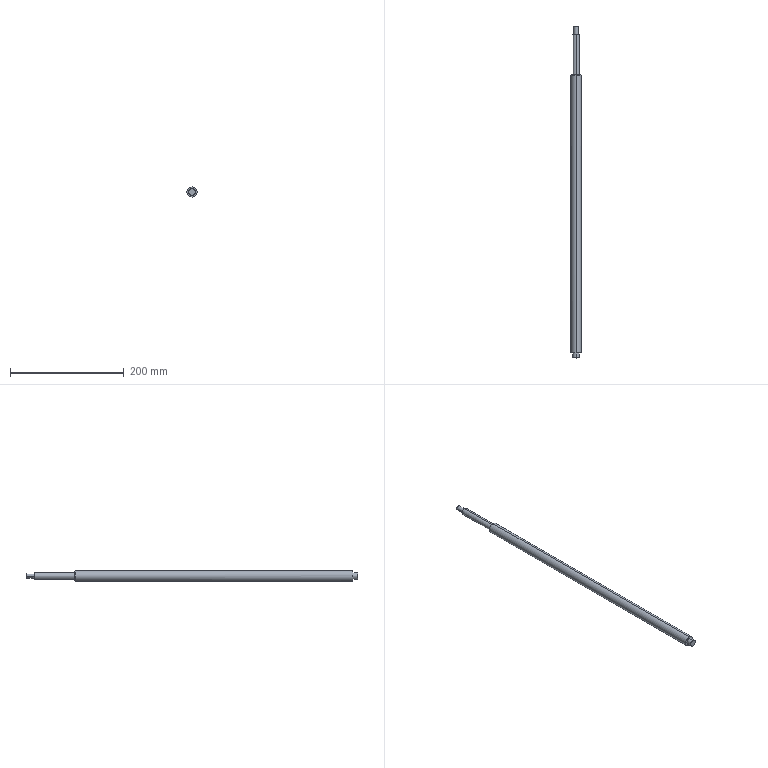Part | SolidWorks | features ICE 4, Chamfer 2, BaseBody 1, Fillet 1, HoleWzd 1 | 1 solid | 31 faces | box 18 x 585 x 18 mm | volume 134308 mm3 | cylinder 12 | cone 11 | plane 8 | commonest cylinder face diameters 12 x4 3 x2 3.3 x2 8 x2 18 x2
STEP:
#1=CARTESIAN_POINT('',(0.,0.5,6.));
#2=VERTEX_POINT('',#1);
#3=CARTESIAN_POINT('',(0.,0.5,-6.));
#4=VERTEX_POINT('',#3);
#5=CARTESIAN_POINT('',(0.,0.5,0.));
#6=DIRECTION('',(0.,1.,0.));
#7=DIRECTION('',(0.,0.,1.));
#8=AXIS2_PLACEMENT_3D('',#5,#6,#7);
#9=CIRCLE('',#8,6.);
#10=EDGE_CURVE('',#2,#4,#9,.T.);
#11=ORIENTED_EDGE('',*,*,#10,.T.);
#12=CARTESIAN_POINT('',(0.,9.,-6.));
#13=VERTEX_POINT('',#12);
#14=CARTESIAN_POINT('',(0.,0.,-6.));
#15=DIRECTION('',(0.,1.,0.));
#16=VECTOR('',#15,1000.);
#17=LINE('',#14,#16);
#18=EDGE_CURVE('',#4,#13,#17,.T.);
#19=ORIENTED_EDGE('',*,*,#18,.T.);
#20=CARTESIAN_POINT('',(0.,9.,6.));
#21=VERTEX_POINT('',#20);
#22=CARTESIAN_POINT('',(0.,9.,0.));
#23=DIRECTION('',(0.,-1.,0.));
#24=DIRECTION('',(0.,0.,-1.));
#25=AXIS2_PLACEMENT_3D('',#22,#23,#24);
#26=CIRCLE('',#25,6.);
#27=EDGE_CURVE('',#13,#21,#26,.T.);
#28=ORIENTED_EDGE('',*,*,#27,.T.);
#29=CARTESIAN_POINT('',(0.,0.,6.));
#30=DIRECTION('',(0.,1.,0.));
#31=VECTOR('',#30,1000.);
#32=LINE('',#29,#31);
#33=EDGE_CURVE('',#2,#21,#32,.T.);
#34=ORIENTED_EDGE('',*,*,#33,.F.);
#35=EDGE_LOOP('',(#11,#19,#28,#34));
#36=FACE_OUTER_BOUND('',#35,.T.);
#37=CARTESIAN_POINT('',(0.,0.,0.));
#38=DIRECTION('',(0.,1.,0.));
#39=DIRECTION('',(0.,0.,1.));
#40=AXIS2_PLACEMENT_3D('',#37,#38,#39);
#41=CYLINDRICAL_SURFACE('',#40,6.);
#42=ADVANCED_FACE('',(#36),#41,.T.);
#43=CARTESIAN_POINT('',(0.,0.,5.5));
#44=VERTEX_POINT('',#43);
#45=CARTESIAN_POINT('',(0.,0.,-5.5));
#46=VERTEX_POINT('',#45);
#47=CARTESIAN_POINT('',(0.,0.,0.));
#48=DIRECTION('',(0.,1.,0.));
#49=DIRECTION('',(0.,0.,1.));
#50=AXIS2_PLACEMENT_3D('',#47,#48,#49);
#51=CIRCLE('',#50,5.5);
#52=EDGE_CURVE('',#44,#46,#51,.T.);
#53=ORIENTED_EDGE('',*,*,#52,.T.);
#54=CARTESIAN_POINT('',(0.,0.5,-6.));
#55=DIRECTION('',(0.,0.7071,-0.7071));
#56=VECTOR('',#55,1000.);
#57=LINE('',#54,#56);
#58=EDGE_CURVE('',#46,#4,#57,.T.);
#59=ORIENTED_EDGE('',*,*,#58,.T.);
#60=ORIENTED_EDGE('',*,*,#10,.F.);
#61=CARTESIAN_POINT('',(0.,0.5,6.));
#62=DIRECTION('',(0.,0.7071,0.7071));
#63=VECTOR('',#62,1000.);
#64=LINE('',#61,#63);
#65=EDGE_CURVE('',#44,#2,#64,.T.);
#66=ORIENTED_EDGE('',*,*,#65,.F.);
#67=EDGE_LOOP('',(#53,#59,#60,#66));
#68=FACE_OUTER_BOUND('',#67,.T.);
#69=CARTESIAN_POINT('',(0.,0.5,0.));
#70=DIRECTION('',(0.,1.,0.));
#71=DIRECTION('',(0.,0.,1.));
#72=AXIS2_PLACEMENT_3D('',#69,#70,#71);
#73=CONICAL_SURFACE('',#72,6.,0.7854);
#74=ADVANCED_FACE('',(#68),#73,.T.);
#75=CARTESIAN_POINT('',(-3.5,585.,0.));
#76=VERTEX_POINT('',#75);
#77=CARTESIAN_POINT('',(3.5,585.,0.));
#78=VERTEX_POINT('',#77);
#79=CARTESIAN_POINT('',(0.,585.,0.));
#80=DIRECTION('',(0.,1.,0.));
#81=DIRECTION('',(-1.,0.,0.));
#82=AXIS2_PLACEMENT_3D('',#79,#80,#81);
#83=CIRCLE('',#82,3.5);
#84=EDGE_CURVE('',#76,#78,#83,.T.);
#85=ORIENTED_EDGE('',*,*,#84,.F.);
#86=CARTESIAN_POINT('',(-4.,584.5,0.));
#87=VERTEX_POINT('',#86);
#88=CARTESIAN_POINT('',(-3.5,585.,0.));
#89=DIRECTION('',(-0.7071,-0.7071,0.));
#90=VECTOR('',#89,1000.);
#91=LINE('',#88,#90);
#92=EDGE_CURVE('',#76,#87,#91,.T.);
#93=ORIENTED_EDGE('',*,*,#92,.T.);
#94=CARTESIAN_POINT('',(4.,584.5,0.));
#95=VERTEX_POINT('',#94);
#96=CARTESIAN_POINT('',(0.,584.5,0.));
#97=DIRECTION('',(0.,-1.,0.));
#98=DIRECTION('',(-1.,0.,0.));
#99=AXIS2_PLACEMENT_3D('',#96,#97,#98);
#100=CIRCLE('',#99,4.);
#101=EDGE_CURVE('',#95,#87,#100,.T.);
#102=ORIENTED_EDGE('',*,*,#101,.F.);
#103=CARTESIAN_POINT('',(3.5,585.,0.));
#104=DIRECTION('',(0.7071,-0.7071,0.));
#105=VECTOR('',#104,1000.);
#106=LINE('',#103,#105);
#107=EDGE_CURVE('',#78,#95,#106,.T.);
#108=ORIENTED_EDGE('',*,*,#107,.F.);
#109=EDGE_LOOP('',(#85,#93,#102,#108));
#110=FACE_OUTER_BOUND('',#109,.T.);
#111=CARTESIAN_POINT('',(0.,585.,0.));
#112=DIRECTION('',(0.,-1.,0.));
#113=DIRECTION('',(1.,0.,0.));
#114=AXIS2_PLACEMENT_3D('',#111,#112,#113);
#115=CONICAL_SURFACE('',#114,3.5,0.7854);
#116=ADVANCED_FACE('',(#110),#115,.T.);
#117=CARTESIAN_POINT('',(1.5,585.,-3.162));
#118=VERTEX_POINT('',#117);
#119=CARTESIAN_POINT('',(0.,585.,0.));
#120=DIRECTION('',(0.,1.,0.));
#121=DIRECTION('',(-1.,0.,0.));
#122=AXIS2_PLACEMENT_3D('',#119,#120,#121);
#123=CIRCLE('',#122,3.5);
#124=EDGE_CURVE('',#78,#118,#123,.T.);
#125=ORIENTED_EDGE('',*,*,#124,.F.);
#126=ORIENTED_EDGE('',*,*,#107,.T.);
#127=CARTESIAN_POINT('',(1.5,584.5,-3.708));
#128=VERTEX_POINT('',#127);
#129=CARTESIAN_POINT('',(0.,584.5,0.));
#130=DIRECTION('',(0.,-1.,0.));
#131=DIRECTION('',(-1.,0.,0.));
#132=AXIS2_PLACEMENT_3D('',#129,#130,#131);
#133=CIRCLE('',#132,4.);
#134=EDGE_CURVE('',#128,#95,#133,.T.);
#135=ORIENTED_EDGE('',*,*,#134,.F.);
#136=CARTESIAN_POINT('',(1.5,585.,-3.162));
#137=CARTESIAN_POINT('',(1.5,584.835,-3.345));
#138=CARTESIAN_POINT('',(1.5,584.668,-3.527));
#139=CARTESIAN_POINT('',(1.5,584.5,-3.708));
#140=B_SPLINE_CURVE_WITH_KNOTS('',3,(#136,#137,#138,#139),.UNSPECIFIED.,.F.,.F.,(4,4),(0.,0.0007402),.UNSPECIFIED.);
#141=EDGE_CURVE('',#118,#128,#140,.T.);
#142=ORIENTED_EDGE('',*,*,#141,.F.);
#143=EDGE_LOOP('',(#125,#126,#135,#142));
#144=FACE_OUTER_BOUND('',#143,.T.);
#145=CARTESIAN_POINT('',(0.,585.,0.));
#146=DIRECTION('',(0.,-1.,0.));
#147=DIRECTION('',(1.,0.,0.));
#148=AXIS2_PLACEMENT_3D('',#145,#146,#147);
#149=CONICAL_SURFACE('',#148,3.5,0.7854);
#150=ADVANCED_FACE('',(#144),#149,.T.);
#151=CARTESIAN_POINT('',(0.,570.,5.5));
#152=VERTEX_POINT('',#151);
#153=CARTESIAN_POINT('',(0.,570.,-5.5));
#154=VERTEX_POINT('',#153);
#155=CARTESIAN_POINT('',(0.,570.,0.));
#156=DIRECTION('',(0.,1.,0.));
#157=DIRECTION('',(-1.,0.,0.));
#158=AXIS2_PLACEMENT_3D('',#155,#156,#157);
#159=CIRCLE('',#158,5.5);
#160=EDGE_CURVE('',#152,#154,#159,.T.);
#161=ORIENTED_EDGE('',*,*,#160,.F.);
#162=CARTESIAN_POINT('',(0.,569.5,6.));
#163=VERTEX_POINT('',#162);
#164=CARTESIAN_POINT('',(0.,570.,5.5));
#165=DIRECTION('',(0.,-0.7071,0.7071));
#166=VECTOR('',#165,1000.);
#167=LINE('',#164,#166);
#168=EDGE_CURVE('',#152,#163,#167,.T.);
#169=ORIENTED_EDGE('',*,*,#168,.T.);
#170=CARTESIAN_POINT('',(0.,569.5,-6.));
#171=VERTEX_POINT('',#170);
#172=CARTESIAN_POINT('',(0.,569.5,0.));
#173=DIRECTION('',(0.,-1.,0.));
#174=DIRECTION('',(0.,0.,1.));
#175=AXIS2_PLACEMENT_3D('',#172,#173,#174);
#176=CIRCLE('',#175,6.);
#177=EDGE_CURVE('',#171,#163,#176,.T.);
#178=ORIENTED_EDGE('',*,*,#177,.F.);
#179=CARTESIAN_POINT('',(0.,570.,-5.5));
#180=DIRECTION('',(0.,-0.7071,-0.7071));
#181=VECTOR('',#180,1000.);
#182=LINE('',#179,#181);
#183=EDGE_CURVE('',#154,#171,#182,.T.);
#184=ORIENTED_EDGE('',*,*,#183,.F.);
#185=EDGE_LOOP('',(#161,#169,#178,#184));
#186=FACE_OUTER_BOUND('',#185,.T.);
#187=CARTESIAN_POINT('',(0.,570.,0.));
#188=DIRECTION('',(0.,-1.,0.));
#189=DIRECTION('',(0.,0.,-1.));
#190=AXIS2_PLACEMENT_3D('',#187,#188,#189);
#191=CONICAL_SURFACE('',#190,5.5,0.7854);
#192=ADVANCED_FACE('',(#186),#191,.T.);
#193=CARTESIAN_POINT('',(0.,572.9,-1.65));
#194=VERTEX_POINT('',#193);
#195=CARTESIAN_POINT('',(0.,572.9,1.65));
#196=VERTEX_POINT('',#195);
#197=CARTESIAN_POINT('',(0.,572.9,0.));
#198=DIRECTION('',(0.,1.,0.));
#199=DIRECTION('',(0.,0.,1.));
#200=AXIS2_PLACEMENT_3D('',#197,#198,#199);
#201=CIRCLE('',#200,1.65);
#202=EDGE_CURVE('',#194,#196,#201,.T.);
#203=ORIENTED_EDGE('',*,*,#202,.F.);
#204=CARTESIAN_POINT('',(0.,585.,-1.65));
#205=VERTEX_POINT('',#204);
#206=CARTESIAN_POINT('',(0.,585.,-1.65));
#207=DIRECTION('',(0.,1.,0.));
#208=VECTOR('',#207,1000.);
#209=LINE('',#206,#208);
#210=EDGE_CURVE('',#194,#205,#209,.T.);
#211=ORIENTED_EDGE('',*,*,#210,.T.);
#212=CARTESIAN_POINT('',(0.,585.,1.65));
#213=VERTEX_POINT('',#212);
#214=CARTESIAN_POINT('',(0.,585.,0.));
#215=DIRECTION('',(0.,1.,0.));
#216=DIRECTION('',(0.,0.,1.));
#217=AXIS2_PLACEMENT_3D('',#214,#215,#216);
#218=CIRCLE('',#217,1.65);
#219=EDGE_CURVE('',#205,#213,#218,.T.);
#220=ORIENTED_EDGE('',*,*,#219,.T.);
#221=CARTESIAN_POINT('',(0.,585.,1.65));
#222=DIRECTION('',(0.,1.,0.));
#223=VECTOR('',#222,1000.);
#224=LINE('',#221,#223);
#225=EDGE_CURVE('',#196,#213,#224,.T.);
#226=ORIENTED_EDGE('',*,*,#225,.F.);
#227=EDGE_LOOP('',(#203,#211,#220,#226));
#228=FACE_OUTER_BOUND('',#227,.T.);
#229=CARTESIAN_POINT('',(0.,585.,0.));
#230=DIRECTION('',(0.,1.,0.));
#231=DIRECTION('',(0.,0.,1.));
#232=AXIS2_PLACEMENT_3D('',#229,#230,#231);
#233=CYLINDRICAL_SURFACE('',#232,1.65);
#234=ADVANCED_FACE('',(#228),#233,.F.);
#235=CARTESIAN_POINT('',(0.,571.909,0.));
#236=VERTEX_POINT('',#235);
#237=CARTESIAN_POINT('',(0.,572.9,1.65));
#238=DIRECTION('',(0.,0.515,0.8572));
#239=VECTOR('',#238,1000.);
#240=LINE('',#237,#239);
#241=EDGE_CURVE('',#236,#196,#240,.T.);
#242=ORIENTED_EDGE('',*,*,#241,.F.);
#243=CARTESIAN_POINT('',(0.,572.9,-1.65));
#244=DIRECTION('',(0.,0.515,-0.8572));
#245=VECTOR('',#244,1000.);
#246=LINE('',#243,#245);
#247=EDGE_CURVE('',#236,#194,#246,.T.);
#248=ORIENTED_EDGE('',*,*,#247,.T.);
#249=ORIENTED_EDGE('',*,*,#202,.T.);
#250=EDGE_LOOP('',(#242,#248,#249));
#251=FACE_OUTER_BOUND('',#250,.T.);
#252=CARTESIAN_POINT('',(0.,572.9,0.));
#253=DIRECTION('',(0.,1.,0.));
#254=DIRECTION('',(0.,0.,1.));
#255=AXIS2_PLACEMENT_3D('',#252,#253,#254);
#256=CONICAL_SURFACE('',#255,1.65,1.03);
#257=ADVANCED_FACE('',(#251),#256,.F.);
#258=ORIENTED_EDGE('',*,*,#101,.T.);
#259=CARTESIAN_POINT('',(-4.,570.,0.));
#260=VERTEX_POINT('',#259);
#261=CARTESIAN_POINT('',(-4.,585.,0.));
#262=DIRECTION('',(0.,-1.,0.));
#263=VECTOR('',#262,1000.);
#264=LINE('',#261,#263);
#265=EDGE_CURVE('',#87,#260,#264,.T.);
#266=ORIENTED_EDGE('',*,*,#265,.T.);
#267=CARTESIAN_POINT('',(4.,570.,0.));
#268=VERTEX_POINT('',#267);
#269=CARTESIAN_POINT('',(0.,570.,0.));
#270=DIRECTION('',(0.,1.,0.));
#271=DIRECTION('',(-1.,0.,0.));
#272=AXIS2_PLACEMENT_3D('',#269,#270,#271);
#273=CIRCLE('',#272,4.);
#274=EDGE_CURVE('',#260,#268,#273,.T.);
#275=ORIENTED_EDGE('',*,*,#274,.T.);
#276=CARTESIAN_POINT('',(4.,585.,0.));
#277=DIRECTION('',(0.,-1.,0.));
#278=VECTOR('',#277,1000.);
#279=LINE('',#276,#278);
#280=EDGE_CURVE('',#95,#268,#279,.T.);
#281=ORIENTED_EDGE('',*,*,#280,.F.);
#282=EDGE_LOOP('',(#258,#266,#275,#281));
#283=FACE_OUTER_BOUND('',#282,.T.);
#284=CARTESIAN_POINT('',(0.,585.,0.));
#285=DIRECTION('',(0.,-1.,0.));
#286=DIRECTION('',(1.,0.,0.));
#287=AXIS2_PLACEMENT_3D('',#284,#285,#286);
#288=CYLINDRICAL_SURFACE('',#287,4.);
#289=ADVANCED_FACE('',(#283),#288,.T.);
#290=CARTESIAN_POINT('',(8.5,499.,0.));
#291=VERTEX_POINT('',#290);
#292=CARTESIAN_POINT('',(-8.5,499.,0.));
#293=VERTEX_POINT('',#292);
#294=CARTESIAN_POINT('',(0.,499.,0.));
#295=DIRECTION('',(0.,-1.,0.));
#296=DIRECTION('',(1.,0.,0.));
#297=AXIS2_PLACEMENT_3D('',#294,#295,#296);
#298=CIRCLE('',#297,8.5);
#299=EDGE_CURVE('',#291,#293,#298,.T.);
#300=ORIENTED_EDGE('',*,*,#299,.T.);
#301=CARTESIAN_POINT('',(-9.,498.5,0.));
#302=VERTEX_POINT('',#301);
#303=CARTESIAN_POINT('',(-9.,498.5,0.));
#304=DIRECTION('',(-0.7071,-0.7071,0.));
#305=VECTOR('',#304,1000.);
#306=LINE('',#303,#305);
#307=EDGE_CURVE('',#293,#302,#306,.T.);
#308=ORIENTED_EDGE('',*,*,#307,.T.);
#309=CARTESIAN_POINT('',(0.,498.5,9.));
#310=VERTEX_POINT('',#309);
#311=CARTESIAN_POINT('',(0.,498.5,0.));
#312=DIRECTION('',(0.,-1.,0.));
#313=DIRECTION('',(0.,0.,1.));
#314=AXIS2_PLACEMENT_3D('',#311,#312,#313);
#315=CIRCLE('',#314,9.);
#316=EDGE_CURVE('',#310,#302,#315,.T.);
#317=ORIENTED_EDGE('',*,*,#316,.F.);
#318=CARTESIAN_POINT('',(9.,498.5,0.));
#319=VERTEX_POINT('',#318);
#320=CARTESIAN_POINT('',(0.,498.5,0.));
#321=DIRECTION('',(0.,-1.,0.));
#322=DIRECTION('',(0.,0.,1.));
#323=AXIS2_PLACEMENT_3D('',#320,#321,#322);
#324=CIRCLE('',#323,9.);
#325=EDGE_CURVE('',#319,#310,#324,.T.);
#326=ORIENTED_EDGE('',*,*,#325,.F.);
#327=CARTESIAN_POINT('',(9.,498.5,0.));
#328=DIRECTION('',(0.7071,-0.7071,0.));
#329=VECTOR('',#328,1000.);
#330=LINE('',#327,#329);
#331=EDGE_CURVE('',#291,#319,#330,.T.);
#332=ORIENTED_EDGE('',*,*,#331,.F.);
#333=EDGE_LOOP('',(#300,#308,#317,#326,#332));
#334=FACE_OUTER_BOUND('',#333,.T.);
#335=CARTESIAN_POINT('',(0.,498.5,0.));
#336=DIRECTION('',(0.,-1.,0.));
#337=DIRECTION('',(1.,0.,0.));
#338=AXIS2_PLACEMENT_3D('',#335,#336,#337);
#339=CONICAL_SURFACE('',#338,9.,0.7854);
#340=ADVANCED_FACE('',(#334),#339,.T.);
#341=CARTESIAN_POINT('',(0.,499.,-6.));
#342=VERTEX_POINT('',#341);
#343=CARTESIAN_POINT('',(0.,499.,6.));
#344=VERTEX_POINT('',#343);
#345=CARTESIAN_POINT('',(0.,499.,0.));
#346=DIRECTION('',(0.,-1.,0.));
#347=DIRECTION('',(0.,0.,1.));
#348=AXIS2_PLACEMENT_3D('',#345,#346,#347);
#349=CIRCLE('',#348,6.);
#350=EDGE_CURVE('',#342,#344,#349,.T.);
#351=ORIENTED_EDGE('',*,*,#350,.F.);
#352=CARTESIAN_POINT('',(0.,499.,-6.));
#353=DIRECTION('',(0.,1.,0.));
#354=VECTOR('',#353,1000.);
#355=LINE('',#352,#354);
#356=EDGE_CURVE('',#342,#171,#355,.T.);
#357=ORIENTED_EDGE('',*,*,#356,.T.);
#358=ORIENTED_EDGE('',*,*,#177,.T.);
#359=CARTESIAN_POINT('',(0.,499.,6.));
#360=DIRECTION('',(0.,1.,0.));
#361=VECTOR('',#360,1000.);
#362=LINE('',#359,#361);
#363=EDGE_CURVE('',#344,#163,#362,.T.);
#364=ORIENTED_EDGE('',*,*,#363,.F.);
#365=EDGE_LOOP('',(#351,#357,#358,#364));
#366=FACE_OUTER_BOUND('',#365,.T.);
#367=CARTESIAN_POINT('',(0.,499.,0.));
#368=DIRECTION('',(0.,1.,0.));
#369=DIRECTION('',(0.,0.,1.));
#370=AXIS2_PLACEMENT_3D('',#367,#368,#369);
#371=CYLINDRICAL_SURFACE('',#370,6.);
#372=ADVANCED_FACE('',(#366),#371,.T.);
#373=CARTESIAN_POINT('',(0.,9.,-9.));
#374=VERTEX_POINT('',#373);
#375=CARTESIAN_POINT('',(0.,9.,9.));
#376=VERTEX_POINT('',#375);
#377=CARTESIAN_POINT('',(0.,9.,0.));
#378=DIRECTION('',(0.,-1.,0.));
#379=DIRECTION('',(0.,0.,-1.));
#380=AXIS2_PLACEMENT_3D('',#377,#378,#379);
#381=CIRCLE('',#380,9.);
#382=EDGE_CURVE('',#374,#376,#381,.T.);
#383=ORIENTED_EDGE('',*,*,#382,.F.);
#384=CARTESIAN_POINT('',(0.,498.5,-9.));
#385=VERTEX_POINT('',#384);
#386=CARTESIAN_POINT('',(0.,8.,-9.));
#387=DIRECTION('',(0.,1.,0.));
#388=VECTOR('',#387,1000.);
#389=LINE('',#386,#388);
#390=EDGE_CURVE('',#374,#385,#389,.T.);
#391=ORIENTED_EDGE('',*,*,#390,.T.);
#392=CARTESIAN_POINT('',(0.,498.5,0.));
#393=DIRECTION('',(0.,-1.,0.));
#394=DIRECTION('',(0.,0.,1.));
#395=AXIS2_PLACEMENT_3D('',#392,#393,#394);
#396=CIRCLE('',#395,9.);
#397=EDGE_CURVE('',#385,#319,#396,.T.);
#398=ORIENTED_EDGE('',*,*,#397,.T.);
#399=ORIENTED_EDGE('',*,*,#325,.T.);
#400=CARTESIAN_POINT('',(0.,8.,9.));
#401=DIRECTION('',(0.,1.,0.));
#402=VECTOR('',#401,1000.);
#403=LINE('',#400,#402);
#404=EDGE_CURVE('',#376,#310,#403,.T.);
#405=ORIENTED_EDGE('',*,*,#404,.F.);
#406=EDGE_LOOP('',(#383,#391,#398,#399,#405));
#407=FACE_OUTER_BOUND('',#406,.T.);
#408=CARTESIAN_POINT('',(0.,8.,0.));
#409=DIRECTION('',(0.,1.,0.));
#410=DIRECTION('',(0.,0.,1.));
#411=AXIS2_PLACEMENT_3D('',#408,#409,#410);
#412=CYLINDRICAL_SURFACE('',#411,9.);
#413=ADVANCED_FACE('',(#407),#412,.T.);
#414=ORIENTED_EDGE('',*,*,#390,.F.);
#415=CARTESIAN_POINT('',(0.,9.,0.));
#416=DIRECTION('',(0.,-1.,0.));
#417=DIRECTION('',(0.,0.,-1.));
#418=AXIS2_PLACEMENT_3D('',#415,#416,#417);
#419=CIRCLE('',#418,9.);
#420=EDGE_CURVE('',#376,#374,#419,.T.);
#421=ORIENTED_EDGE('',*,*,#420,.F.);
#422=ORIENTED_EDGE('',*,*,#404,.T.);
#423=ORIENTED_EDGE('',*,*,#316,.T.);
#424=CARTESIAN_POINT('',(0.,498.5,0.));
#425=DIRECTION('',(0.,-1.,0.));
#426=DIRECTION('',(0.,0.,1.));
#427=AXIS2_PLACEMENT_3D('',#424,#425,#426);
#428=CIRCLE('',#427,9.);
#429=EDGE_CURVE('',#302,#385,#428,.T.);
#430=ORIENTED_EDGE('',*,*,#429,.T.);
#431=EDGE_LOOP('',(#414,#421,#422,#423,#430));
#432=FACE_OUTER_BOUND('',#431,.T.);
#433=CARTESIAN_POINT('',(0.,8.,0.));
#434=DIRECTION('',(0.,1.,0.));
#435=DIRECTION('',(0.,0.,1.));
#436=AXIS2_PLACEMENT_3D('',#433,#434,#435);
#437=CYLINDRICAL_SURFACE('',#436,9.);
#438=ADVANCED_FACE('',(#432),#437,.T.);
#439=CARTESIAN_POINT('',(0.,570.,0.));
#440=DIRECTION('',(0.,1.,0.));
#441=DIRECTION('',(-1.,0.,0.));
#442=AXIS2_PLACEMENT_3D('',#439,#440,#441);
#443=CIRCLE('',#442,5.5);
#444=EDGE_CURVE('',#154,#152,#443,.T.);
#445=ORIENTED_EDGE('',*,*,#444,.T.);
#446=ORIENTED_EDGE('',*,*,#160,.T.);
#447=EDGE_LOOP('',(#445,#446));
#448=FACE_OUTER_BOUND('',#447,.T.);
#449=CARTESIAN_POINT('',(0.,570.,0.));
#450=DIRECTION('',(0.,1.,0.));
#451=DIRECTION('',(-1.,0.,0.));
#452=AXIS2_PLACEMENT_3D('',#449,#450,#451);
#453=CIRCLE('',#452,4.);
#454=EDGE_CURVE('',#268,#260,#453,.T.);
#455=ORIENTED_EDGE('',*,*,#454,.F.);
#456=ORIENTED_EDGE('',*,*,#274,.F.);
#457=EDGE_LOOP('',(#455,#456));
#458=FACE_BOUND('',#457,.T.);
#459=CARTESIAN_POINT('',(0.,570.,0.));
#460=DIRECTION('',(0.,1.,0.));
#461=DIRECTION('',(-1.,0.,0.));
#462=AXIS2_PLACEMENT_3D('',#459,#460,#461);
#463=PLANE('',#462);
#464=ADVANCED_FACE('',(#448,#458),#463,.T.);
#465=ORIENTED_EDGE('',*,*,#307,.F.);
#466=CARTESIAN_POINT('',(0.,499.,0.));
#467=DIRECTION('',(0.,-1.,0.));
#468=DIRECTION('',(1.,0.,0.));
#469=AXIS2_PLACEMENT_3D('',#466,#467,#468);
#470=CIRCLE('',#469,8.5);
#471=EDGE_CURVE('',#293,#291,#470,.T.);
#472=ORIENTED_EDGE('',*,*,#471,.T.);
#473=ORIENTED_EDGE('',*,*,#331,.T.);
#474=ORIENTED_EDGE('',*,*,#397,.F.);
#475=ORIENTED_EDGE('',*,*,#429,.F.);
#476=EDGE_LOOP('',(#465,#472,#473,#474,#475));
#477=FACE_OUTER_BOUND('',#476,.T.);
#478=CARTESIAN_POINT('',(0.,498.5,0.));
#479=DIRECTION('',(0.,-1.,0.));
#480=DIRECTION('',(1.,0.,0.));
#481=AXIS2_PLACEMENT_3D('',#478,#479,#480);
#482=CONICAL_SURFACE('',#481,9.,0.7854);
#483=ADVANCED_FACE('',(#477),#482,.T.);
#484=CARTESIAN_POINT('',(0.,499.,0.));
#485=DIRECTION('',(0.,-1.,0.));
#486=DIRECTION('',(0.,0.,1.));
#487=AXIS2_PLACEMENT_3D('',#484,#485,#486);
#488=CIRCLE('',#487,6.);
#489=EDGE_CURVE('',#344,#342,#488,.T.);
#490=ORIENTED_EDGE('',*,*,#489,.T.);
#491=ORIENTED_EDGE('',*,*,#350,.T.);
#492=EDGE_LOOP('',(#490,#491));
#493=FACE_BOUND('',#492,.T.);
#494=ORIENTED_EDGE('',*,*,#299,.F.);
#495=ORIENTED_EDGE('',*,*,#471,.F.);
#496=EDGE_LOOP('',(#494,#495));
#497=FACE_OUTER_BOUND('',#496,.T.);
#498=CARTESIAN_POINT('',(0.,499.,0.));
#499=DIRECTION('',(0.,1.,0.));
#500=DIRECTION('',(0.,0.,1.));
#501=AXIS2_PLACEMENT_3D('',#498,#499,#500);
#502=PLANE('',#501);
#503=ADVANCED_FACE('',(#493,#497),#502,.T.);
#504=ORIENTED_EDGE('',*,*,#356,.F.);
#505=ORIENTED_EDGE('',*,*,#489,.F.);
#506=ORIENTED_EDGE('',*,*,#363,.T.);
#507=CARTESIAN_POINT('',(0.,569.5,0.));
#508=DIRECTION('',(0.,-1.,0.));
#509=DIRECTION('',(0.,0.,1.));
#510=AXIS2_PLACEMENT_3D('',#507,#508,#509);
#511=CIRCLE('',#510,6.);
#512=EDGE_CURVE('',#163,#171,#511,.T.);
#513=ORIENTED_EDGE('',*,*,#512,.T.);
#514=EDGE_LOOP('',(#504,#505,#506,#513));
#515=FACE_OUTER_BOUND('',#514,.T.);
#516=CARTESIAN_POINT('',(0.,499.,0.));
#517=DIRECTION('',(0.,1.,0.));
#518=DIRECTION('',(0.,0.,1.));
#519=AXIS2_PLACEMENT_3D('',#516,#517,#518);
#520=CYLINDRICAL_SURFACE('',#519,6.);
#521=ADVANCED_FACE('',(#515),#520,.T.);
#522=ORIENTED_EDGE('',*,*,#265,.F.);
#523=CARTESIAN_POINT('',(-1.5,584.5,-3.708));
#524=VERTEX_POINT('',#523);
#525=CARTESIAN_POINT('',(0.,584.5,0.));
#526=DIRECTION('',(0.,-1.,0.));
#527=DIRECTION('',(-1.,0.,0.));
#528=AXIS2_PLACEMENT_3D('',#525,#526,#527);
#529=CIRCLE('',#528,4.);
#530=EDGE_CURVE('',#87,#524,#529,.T.);
#531=ORIENTED_EDGE('',*,*,#530,.T.);
#532=CARTESIAN_POINT('',(-1.5,574.,-3.708));
#533=VERTEX_POINT('',#532);
#534=CARTESIAN_POINT('',(-1.5,585.,-3.708));
#535=DIRECTION('',(0.,-1.,0.));
#536=VECTOR('',#535,1000.);
#537=LINE('',#534,#536);
#538=EDGE_CURVE('',#524,#533,#537,.T.);
#539=ORIENTED_EDGE('',*,*,#538,.T.);
#540=CARTESIAN_POINT('',(0.,572.5,-4.));
#541=VERTEX_POINT('',#540);
#542=CARTESIAN_POINT('',(-1.5,574.,-3.708));
#543=CARTESIAN_POINT('',(-1.5,573.9,-3.708));
#544=CARTESIAN_POINT('',(-1.49,573.802,-3.712));
#545=CARTESIAN_POINT('',(-1.451,573.609,-3.727));
#546=CARTESIAN_POINT('',(-1.422,573.513,-3.739));
#547=CARTESIAN_POINT('',(-1.309,573.242,-3.781));
#548=CARTESIAN_POINT('',(-1.198,573.077,-3.819));
#549=CARTESIAN_POINT('',(-0.9242,572.803,-3.894));
#550=CARTESIAN_POINT('',(-0.7585,572.691,-3.932));
#551=CARTESIAN_POINT('',(-0.3984,572.541,-3.984));
#552=CARTESIAN_POINT('',(-0.2001,572.5,-4.));
#553=CARTESIAN_POINT('',(0.,572.5,-4.));
#554=B_SPLINE_CURVE_WITH_KNOTS('',3,(#542,#543,#544,#545,#546,#547,#548,#549,#550,#551,#552,#553),.UNSPECIFIED.,.F.,.F.,(4,2,2,2,2,4),(0.,0.0002956,0.0005913,0.001183,0.001774,0.002365),.UNSPECIFIED.);
#555=EDGE_CURVE('',#533,#541,#554,.T.);
#556=ORIENTED_EDGE('',*,*,#555,.T.);
#557=CARTESIAN_POINT('',(1.5,574.,-3.708));
#558=VERTEX_POINT('',#557);
#559=CARTESIAN_POINT('',(0.,572.5,-4.));
#560=CARTESIAN_POINT('',(0.1,572.5,-4.));
#561=CARTESIAN_POINT('',(0.1982,572.51,-3.996));
#562=CARTESIAN_POINT('',(0.3911,572.549,-3.982));
#563=CARTESIAN_POINT('',(0.4868,572.578,-3.971));
#564=CARTESIAN_POINT('',(0.7587,572.691,-3.932));
#565=CARTESIAN_POINT('',(0.9238,572.802,-3.894));
#566=CARTESIAN_POINT('',(1.198,573.076,-3.819));
#567=CARTESIAN_POINT('',(1.309,573.242,-3.781));
#568=CARTESIAN_POINT('',(1.459,573.602,-3.725));
#569=CARTESIAN_POINT('',(1.5,573.8,-3.708));
#570=CARTESIAN_POINT('',(1.5,574.,-3.708));
#571=B_SPLINE_CURVE_WITH_KNOTS('',3,(#559,#560,#561,#562,#563,#564,#565,#566,#567,#568,#569,#570),.UNSPECIFIED.,.F.,.F.,(4,2,2,2,2,4),(0.,0.0002957,0.0005913,0.001183,0.001774,0.002365),.UNSPECIFIED.);
#572=EDGE_CURVE('',#541,#558,#571,.T.);
#573=ORIENTED_EDGE('',*,*,#572,.T.);
#574=CARTESIAN_POINT('',(1.5,585.,-3.708));
#575=DIRECTION('',(0.,1.,0.));
#576=VECTOR('',#575,1000.);
#577=LINE('',#574,#576);
#578=EDGE_CURVE('',#558,#128,#577,.T.);
#579=ORIENTED_EDGE('',*,*,#578,.T.);
#580=ORIENTED_EDGE('',*,*,#134,.T.);
#581=ORIENTED_EDGE('',*,*,#280,.T.);
#582=ORIENTED_EDGE('',*,*,#454,.T.);
#583=EDGE_LOOP('',(#522,#531,#539,#556,#573,#579,#580,#581,#582));
#584=FACE_OUTER_BOUND('',#583,.T.);
#585=CARTESIAN_POINT('',(0.,585.,0.));
#586=DIRECTION('',(0.,-1.,0.));
#587=DIRECTION('',(1.,0.,0.));
#588=AXIS2_PLACEMENT_3D('',#585,#586,#587);
#589=CYLINDRICAL_SURFACE('',#588,4.);
#590=ADVANCED_FACE('',(#584),#589,.T.);
#591=CARTESIAN_POINT('',(0.,585.,0.));
#592=DIRECTION('',(0.,1.,0.));
#593=DIRECTION('',(0.,0.,1.));
#594=AXIS2_PLACEMENT_3D('',#591,#592,#593);
#595=CIRCLE('',#594,1.65);
#596=EDGE_CURVE('',#213,#205,#595,.T.);
#597=ORIENTED_EDGE('',*,*,#596,.F.);
#598=ORIENTED_EDGE('',*,*,#219,.F.);
#599=EDGE_LOOP('',(#597,#598));
#600=FACE_BOUND('',#599,.T.);
#601=CARTESIAN_POINT('',(-1.5,585.,-3.162));
#602=VERTEX_POINT('',#601);
#603=CARTESIAN_POINT('',(-1.5,585.,-2.3));
#604=VERTEX_POINT('',#603);
#605=CARTESIAN_POINT('',(-1.5,585.,0.));
#606=DIRECTION('',(0.,0.,1.));
#607=VECTOR('',#606,1000.);
#608=LINE('',#605,#607);
#609=EDGE_CURVE('',#602,#604,#608,.T.);
#610=ORIENTED_EDGE('',*,*,#609,.F.);
#611=CARTESIAN_POINT('',(0.,585.,0.));
#612=DIRECTION('',(0.,1.,0.));
#613=DIRECTION('',(-1.,0.,0.));
#614=AXIS2_PLACEMENT_3D('',#611,#612,#613);
#615=CIRCLE('',#614,3.5);
#616=EDGE_CURVE('',#602,#76,#615,.T.);
#617=ORIENTED_EDGE('',*,*,#616,.T.);
#618=ORIENTED_EDGE('',*,*,#84,.T.);
#619=ORIENTED_EDGE('',*,*,#124,.T.);
#620=CARTESIAN_POINT('',(1.5,585.,-2.3));
#621=VERTEX_POINT('',#620);
#622=CARTESIAN_POINT('',(1.5,585.,-4.));
#623=DIRECTION('',(0.,0.,-1.));
#624=VECTOR('',#623,1000.);
#625=LINE('',#622,#624);
#626=EDGE_CURVE('',#621,#118,#625,.T.);
#627=ORIENTED_EDGE('',*,*,#626,.F.);
#628=CARTESIAN_POINT('',(-1.5,585.,-2.3));
#629=DIRECTION('',(1.,0.,0.));
#630=VECTOR('',#629,1000.);
#631=LINE('',#628,#630);
#632=EDGE_CURVE('',#604,#621,#631,.T.);
#633=ORIENTED_EDGE('',*,*,#632,.F.);
#634=EDGE_LOOP('',(#610,#617,#618,#619,#627,#633));
#635=FACE_OUTER_BOUND('',#634,.T.);
#636=CARTESIAN_POINT('',(0.,585.,0.));
#637=DIRECTION('',(0.,1.,0.));
#638=DIRECTION('',(-1.,0.,0.));
#639=AXIS2_PLACEMENT_3D('',#636,#637,#638);
#640=PLANE('',#639);
#641=ADVANCED_FACE('',(#600,#635),#640,.T.);
#642=ORIENTED_EDGE('',*,*,#538,.F.);
#643=CARTESIAN_POINT('',(-1.5,584.5,-3.708));
#644=CARTESIAN_POINT('',(-1.5,584.668,-3.527));
#645=CARTESIAN_POINT('',(-1.5,584.835,-3.345));
#646=CARTESIAN_POINT('',(-1.5,585.,-3.162));
#647=B_SPLINE_CURVE_WITH_KNOTS('',3,(#643,#644,#645,#646),.UNSPECIFIED.,.F.,.F.,(4,4),(0.,0.0007402),.UNSPECIFIED.);
#648=EDGE_CURVE('',#524,#602,#647,.T.);
#649=ORIENTED_EDGE('',*,*,#648,.T.);
#650=ORIENTED_EDGE('',*,*,#609,.T.);
#651=CARTESIAN_POINT('',(-1.5,574.,-2.3));
#652=VERTEX_POINT('',#651);
#653=CARTESIAN_POINT('',(-1.5,572.5,-2.3));
#654=DIRECTION('',(0.,1.,0.));
#655=VECTOR('',#654,1000.);
#656=LINE('',#653,#655);
#657=EDGE_CURVE('',#652,#604,#656,.T.);
#658=ORIENTED_EDGE('',*,*,#657,.F.);
#659=CARTESIAN_POINT('',(-1.5,574.,-4.));
#660=DIRECTION('',(0.,0.,-1.));
#661=VECTOR('',#660,1000.);
#662=LINE('',#659,#661);
#663=EDGE_CURVE('',#652,#533,#662,.T.);
#664=ORIENTED_EDGE('',*,*,#663,.T.);
#665=EDGE_LOOP('',(#642,#649,#650,#658,#664));
#666=FACE_OUTER_BOUND('',#665,.T.);
#667=CARTESIAN_POINT('',(-1.5,572.5,-4.));
#668=DIRECTION('',(-1.,0.,0.));
#669=DIRECTION('',(0.,0.,1.));
#670=AXIS2_PLACEMENT_3D('',#667,#668,#669);
#671=PLANE('',#670);
#672=ADVANCED_FACE('',(#666),#671,.F.);
#673=ORIENTED_EDGE('',*,*,#626,.T.);
#674=ORIENTED_EDGE('',*,*,#141,.T.);
#675=ORIENTED_EDGE('',*,*,#578,.F.);
#676=CARTESIAN_POINT('',(1.5,574.,-2.3));
#677=VERTEX_POINT('',#676);
#678=CARTESIAN_POINT('',(1.5,574.,-4.));
#679=DIRECTION('',(0.,0.,1.));
#680=VECTOR('',#679,1000.);
#681=LINE('',#678,#680);
#682=EDGE_CURVE('',#558,#677,#681,.T.);
#683=ORIENTED_EDGE('',*,*,#682,.T.);
#684=CARTESIAN_POINT('',(1.5,572.5,-2.3));
#685=DIRECTION('',(0.,1.,0.));
#686=VECTOR('',#685,1000.);
#687=LINE('',#684,#686);
#688=EDGE_CURVE('',#677,#621,#687,.T.);
#689=ORIENTED_EDGE('',*,*,#688,.T.);
#690=EDGE_LOOP('',(#673,#674,#675,#683,#689));
#691=FACE_OUTER_BOUND('',#690,.T.);
#692=CARTESIAN_POINT('',(1.5,572.5,-4.));
#693=DIRECTION('',(1.,0.,0.));
#694=DIRECTION('',(0.,0.,-1.));
#695=AXIS2_PLACEMENT_3D('',#692,#693,#694);
#696=PLANE('',#695);
#697=ADVANCED_FACE('',(#691),#696,.F.);
#698=ORIENTED_EDGE('',*,*,#688,.F.);
#699=CARTESIAN_POINT('',(0.,572.5,-2.3));
#700=VERTEX_POINT('',#699);
#701=CARTESIAN_POINT('',(0.,574.,-2.3));
#702=DIRECTION('',(0.,0.,-1.));
#703=DIRECTION('',(1.,0.,0.));
#704=AXIS2_PLACEMENT_3D('',#701,#702,#703);
#705=CIRCLE('',#704,1.5);
#706=EDGE_CURVE('',#677,#700,#705,.T.);
#707=ORIENTED_EDGE('',*,*,#706,.T.);
#708=CARTESIAN_POINT('',(0.,574.,-2.3));
#709=DIRECTION('',(0.,0.,-1.));
#710=DIRECTION('',(1.,0.,0.));
#711=AXIS2_PLACEMENT_3D('',#708,#709,#710);
#712=CIRCLE('',#711,1.5);
#713=EDGE_CURVE('',#700,#652,#712,.T.);
#714=ORIENTED_EDGE('',*,*,#713,.T.);
#715=ORIENTED_EDGE('',*,*,#657,.T.);
#716=ORIENTED_EDGE('',*,*,#632,.T.);
#717=EDGE_LOOP('',(#698,#707,#714,#715,#716));
#718=FACE_OUTER_BOUND('',#717,.T.);
#719=CARTESIAN_POINT('',(-1.5,572.5,-2.3));
#720=DIRECTION('',(0.,0.,1.));
#721=DIRECTION('',(1.,0.,0.));
#722=AXIS2_PLACEMENT_3D('',#719,#720,#721);
#723=PLANE('',#722);
#724=ADVANCED_FACE('',(#718),#723,.F.);
#725=ORIENTED_EDGE('',*,*,#663,.F.);
#726=ORIENTED_EDGE('',*,*,#713,.F.);
#727=CARTESIAN_POINT('',(0.,572.5,-2.3));
#728=DIRECTION('',(0.,0.,1.));
#729=VECTOR('',#728,1000.);
#730=LINE('',#727,#729);
#731=EDGE_CURVE('',#541,#700,#730,.T.);
#732=ORIENTED_EDGE('',*,*,#731,.F.);
#733=ORIENTED_EDGE('',*,*,#555,.F.);
#734=EDGE_LOOP('',(#725,#726,#732,#733));
#735=FACE_OUTER_BOUND('',#734,.T.);
#736=CARTESIAN_POINT('',(0.,574.,-2.3));
#737=DIRECTION('',(0.,0.,1.));
#738=DIRECTION('',(1.,0.,0.));
#739=AXIS2_PLACEMENT_3D('',#736,#737,#738);
#740=CYLINDRICAL_SURFACE('',#739,1.5);
#741=ADVANCED_FACE('',(#735),#740,.F.);
#742=ORIENTED_EDGE('',*,*,#706,.F.);
#743=ORIENTED_EDGE('',*,*,#682,.F.);
#744=ORIENTED_EDGE('',*,*,#572,.F.);
#745=ORIENTED_EDGE('',*,*,#731,.T.);
#746=EDGE_LOOP('',(#742,#743,#744,#745));
#747=FACE_OUTER_BOUND('',#746,.T.);
#748=CARTESIAN_POINT('',(0.,574.,-2.3));
#749=DIRECTION('',(0.,0.,-1.));
#750=DIRECTION('',(-1.,0.,0.));
#751=AXIS2_PLACEMENT_3D('',#748,#749,#750);
#752=CYLINDRICAL_SURFACE('',#751,1.5);
#753=ADVANCED_FACE('',(#747),#752,.F.);
#754=ORIENTED_EDGE('',*,*,#247,.F.);
#755=ORIENTED_EDGE('',*,*,#241,.T.);
#756=CARTESIAN_POINT('',(0.,572.9,0.));
#757=DIRECTION('',(0.,1.,0.));
#758=DIRECTION('',(0.,0.,1.));
#759=AXIS2_PLACEMENT_3D('',#756,#757,#758);
#760=CIRCLE('',#759,1.65);
#761=EDGE_CURVE('',#196,#194,#760,.T.);
#762=ORIENTED_EDGE('',*,*,#761,.T.);
#763=EDGE_LOOP('',(#754,#755,#762));
#764=FACE_OUTER_BOUND('',#763,.T.);
#765=CARTESIAN_POINT('',(0.,572.9,0.));
#766=DIRECTION('',(0.,1.,0.));
#767=DIRECTION('',(0.,0.,1.));
#768=AXIS2_PLACEMENT_3D('',#765,#766,#767);
#769=CONICAL_SURFACE('',#768,1.65,1.03);
#770=ADVANCED_FACE('',(#764),#769,.F.);
#771=ORIENTED_EDGE('',*,*,#210,.F.);
#772=ORIENTED_EDGE('',*,*,#761,.F.);
#773=ORIENTED_EDGE('',*,*,#225,.T.);
#774=ORIENTED_EDGE('',*,*,#596,.T.);
#775=EDGE_LOOP('',(#771,#772,#773,#774));
#776=FACE_OUTER_BOUND('',#775,.T.);
#777=CARTESIAN_POINT('',(0.,585.,0.));
#778=DIRECTION('',(0.,1.,0.));
#779=DIRECTION('',(0.,0.,1.));
#780=AXIS2_PLACEMENT_3D('',#777,#778,#779);
#781=CYLINDRICAL_SURFACE('',#780,1.65);
#782=ADVANCED_FACE('',(#776),#781,.F.);
#783=ORIENTED_EDGE('',*,*,#168,.F.);
#784=ORIENTED_EDGE('',*,*,#444,.F.);
#785=ORIENTED_EDGE('',*,*,#183,.T.);
#786=ORIENTED_EDGE('',*,*,#512,.F.);
#787=EDGE_LOOP('',(#783,#784,#785,#786));
#788=FACE_OUTER_BOUND('',#787,.T.);
#789=CARTESIAN_POINT('',(0.,570.,0.));
#790=DIRECTION('',(0.,-1.,0.));
#791=DIRECTION('',(0.,0.,-1.));
#792=AXIS2_PLACEMENT_3D('',#789,#790,#791);
#793=CONICAL_SURFACE('',#792,5.5,0.7854);
#794=ADVANCED_FACE('',(#788),#793,.T.);
#795=ORIENTED_EDGE('',*,*,#92,.F.);
#796=ORIENTED_EDGE('',*,*,#616,.F.);
#797=ORIENTED_EDGE('',*,*,#648,.F.);
#798=ORIENTED_EDGE('',*,*,#530,.F.);
#799=EDGE_LOOP('',(#795,#796,#797,#798));
#800=FACE_OUTER_BOUND('',#799,.T.);
#801=CARTESIAN_POINT('',(0.,585.,0.));
#802=DIRECTION('',(0.,-1.,0.));
#803=DIRECTION('',(1.,0.,0.));
#804=AXIS2_PLACEMENT_3D('',#801,#802,#803);
#805=CONICAL_SURFACE('',#804,3.5,0.7854);
#806=ADVANCED_FACE('',(#800),#805,.T.);
#807=CARTESIAN_POINT('',(0.,9.,0.));
#808=DIRECTION('',(0.,-1.,0.));
#809=DIRECTION('',(0.,0.,-1.));
#810=AXIS2_PLACEMENT_3D('',#807,#808,#809);
#811=CIRCLE('',#810,6.);
#812=EDGE_CURVE('',#21,#13,#811,.T.);
#813=ORIENTED_EDGE('',*,*,#812,.F.);
#814=ORIENTED_EDGE('',*,*,#27,.F.);
#815=EDGE_LOOP('',(#813,#814));
#816=FACE_BOUND('',#815,.T.);
#817=ORIENTED_EDGE('',*,*,#420,.T.);
#818=ORIENTED_EDGE('',*,*,#382,.T.);
#819=EDGE_LOOP('',(#817,#818));
#820=FACE_OUTER_BOUND('',#819,.T.);
#821=CARTESIAN_POINT('',(0.,9.,0.));
#822=DIRECTION('',(0.,-1.,0.));
#823=DIRECTION('',(0.,0.,-1.));
#824=AXIS2_PLACEMENT_3D('',#821,#822,#823);
#825=PLANE('',#824);
#826=ADVANCED_FACE('',(#816,#820),#825,.T.);
#827=ORIENTED_EDGE('',*,*,#52,.F.);
#828=CARTESIAN_POINT('',(0.,0.,0.));
#829=DIRECTION('',(0.,1.,0.));
#830=DIRECTION('',(0.,0.,1.));
#831=AXIS2_PLACEMENT_3D('',#828,#829,#830);
#832=CIRCLE('',#831,5.5);
#833=EDGE_CURVE('',#46,#44,#832,.T.);
#834=ORIENTED_EDGE('',*,*,#833,.F.);
#835=EDGE_LOOP('',(#827,#834));
#836=FACE_OUTER_BOUND('',#835,.T.);
#837=CARTESIAN_POINT('',(0.,0.,0.));
#838=DIRECTION('',(0.,1.,0.));
#839=DIRECTION('',(0.,0.,1.));
#840=AXIS2_PLACEMENT_3D('',#837,#838,#839);
#841=PLANE('',#840);
#842=ADVANCED_FACE('',(#836),#841,.F.);
#843=ORIENTED_EDGE('',*,*,#58,.F.);
#844=ORIENTED_EDGE('',*,*,#833,.T.);
#845=ORIENTED_EDGE('',*,*,#65,.T.);
#846=CARTESIAN_POINT('',(0.,0.5,0.));
#847=DIRECTION('',(0.,1.,0.));
#848=DIRECTION('',(0.,0.,1.));
#849=AXIS2_PLACEMENT_3D('',#846,#847,#848);
#850=CIRCLE('',#849,6.);
#851=EDGE_CURVE('',#4,#2,#850,.T.);
#852=ORIENTED_EDGE('',*,*,#851,.F.);
#853=EDGE_LOOP('',(#843,#844,#845,#852));
#854=FACE_OUTER_BOUND('',#853,.T.);
#855=CARTESIAN_POINT('',(0.,0.5,0.));
#856=DIRECTION('',(0.,1.,0.));
#857=DIRECTION('',(0.,0.,1.));
#858=AXIS2_PLACEMENT_3D('',#855,#856,#857);
#859=CONICAL_SURFACE('',#858,6.,0.7854);
#860=ADVANCED_FACE('',(#854),#859,.T.);
#861=ORIENTED_EDGE('',*,*,#18,.F.);
#862=ORIENTED_EDGE('',*,*,#851,.T.);
#863=ORIENTED_EDGE('',*,*,#33,.T.);
#864=ORIENTED_EDGE('',*,*,#812,.T.);
#865=EDGE_LOOP('',(#861,#862,#863,#864));
#866=FACE_OUTER_BOUND('',#865,.T.);
#867=CARTESIAN_POINT('',(0.,0.,0.));
#868=DIRECTION('',(0.,1.,0.));
#869=DIRECTION('',(0.,0.,1.));
#870=AXIS2_PLACEMENT_3D('',#867,#868,#869);
#871=CYLINDRICAL_SURFACE('',#870,6.);
#872=ADVANCED_FACE('',(#866),#871,.T.);
#873=CLOSED_SHELL('',(#42,#74,#116,#150,#192,#234,#257,#289,#340,#372,#413,#438,#464,#483,#503,#521,#590,#641,#672,#697,#724,#741,#753,#770,#782,#794,#806,#826,#842,#860,#872));
#874=MANIFOLD_SOLID_BREP('',#873);
#875=CARTESIAN_POINT('',(0.,0.,0.));
#876=DIRECTION('',(0.,0.,1.));
#877=DIRECTION('',(1.,0.,0.));
#878=AXIS2_PLACEMENT_3D('',#875,#876,#877);
#879=(LENGTH_UNIT()NAMED_UNIT(*)SI_UNIT(.MILLI.,.METRE.));
#880=UNCERTAINTY_MEASURE_WITH_UNIT(LENGTH_MEASURE(0.00001),#879,'','');
#881=(NAMED_UNIT(*)PLANE_ANGLE_UNIT()SI_UNIT($,.RADIAN.));
#882=(NAMED_UNIT(*)SI_UNIT($,.STERADIAN.)SOLID_ANGLE_UNIT());
#883=(GEOMETRIC_REPRESENTATION_CONTEXT(3)GLOBAL_UNCERTAINTY_ASSIGNED_CONTEXT((#880))GLOBAL_UNIT_ASSIGNED_CONTEXT((#879,#881,#882))REPRESENTATION_CONTEXT('',''));
#884=ADVANCED_BREP_SHAPE_REPRESENTATION('',(#874,#878),#883);